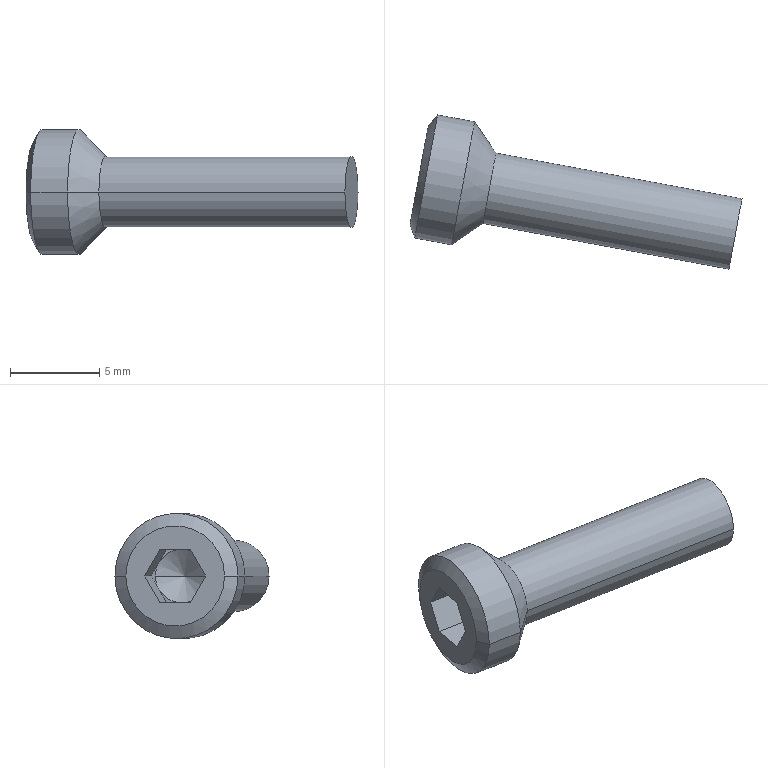Part | SolidWorks | features BaseBody 1 | 1 solid | 24 faces | box 18.575 x 8.622 x 7 mm | volume 288.186 mm3 | plane 14 | cone 6 | cylinder 4 | commonest cylinder face diameters 4 x2 7 x2
STEP:
#1=CARTESIAN_POINT('',(-115.606,1844.083,78.9));
#2=VERTEX_POINT('',#1);
#3=CARTESIAN_POINT('',(-114.875,1848.016,78.9));
#4=VERTEX_POINT('',#3);
#5=CARTESIAN_POINT('',(-115.241,1846.05,78.9));
#6=DIRECTION('',(-0.9832,0.1826,0.));
#7=DIRECTION('',(-0.1826,-0.9832,0.));
#8=AXIS2_PLACEMENT_3D('',#5,#6,#7);
#9=CIRCLE('',#8,2.);
#10=EDGE_CURVE('',#2,#4,#9,.T.);
#11=ORIENTED_EDGE('',*,*,#10,.T.);
#12=CARTESIAN_POINT('',(-128.64,1850.573,78.9));
#13=VERTEX_POINT('',#12);
#14=CARTESIAN_POINT('',(-132.573,1851.303,78.9));
#15=DIRECTION('',(-0.9832,0.1826,0.));
#16=VECTOR('',#15,1000.);
#17=LINE('',#14,#16);
#18=EDGE_CURVE('',#4,#13,#17,.T.);
#19=ORIENTED_EDGE('',*,*,#18,.T.);
#20=CARTESIAN_POINT('',(-129.37,1846.64,78.9));
#21=VERTEX_POINT('',#20);
#22=CARTESIAN_POINT('',(-129.005,1848.607,78.9));
#23=DIRECTION('',(0.9832,-0.1826,0.));
#24=DIRECTION('',(-0.1826,-0.9832,0.));
#25=AXIS2_PLACEMENT_3D('',#22,#23,#24);
#26=CIRCLE('',#25,2.);
#27=EDGE_CURVE('',#13,#21,#26,.T.);
#28=ORIENTED_EDGE('',*,*,#27,.T.);
#29=CARTESIAN_POINT('',(-133.303,1847.371,78.9));
#30=DIRECTION('',(-0.9832,0.1826,0.));
#31=VECTOR('',#30,1000.);
#32=LINE('',#29,#31);
#33=EDGE_CURVE('',#2,#21,#32,.T.);
#34=ORIENTED_EDGE('',*,*,#33,.F.);
#35=EDGE_LOOP('',(#11,#19,#28,#34));
#36=FACE_OUTER_BOUND('',#35,.T.);
#37=CARTESIAN_POINT('',(-132.938,1849.337,78.9));
#38=DIRECTION('',(-0.9832,0.1826,0.));
#39=DIRECTION('',(-0.1826,-0.9832,0.));
#40=AXIS2_PLACEMENT_3D('',#37,#38,#39);
#41=CYLINDRICAL_SURFACE('',#40,2.);
#42=ADVANCED_FACE('',(#36),#41,.T.);
#43=ORIENTED_EDGE('',*,*,#27,.F.);
#44=CARTESIAN_POINT('',(-129.841,1852.322,78.9));
#45=VERTEX_POINT('',#44);
#46=CARTESIAN_POINT('',(-129.841,1852.322,78.9));
#47=DIRECTION('',(-0.5661,0.8244,0.));
#48=VECTOR('',#47,1000.);
#49=LINE('',#46,#48);
#50=EDGE_CURVE('',#13,#45,#49,.T.);
#51=ORIENTED_EDGE('',*,*,#50,.T.);
#52=CARTESIAN_POINT('',(-131.119,1845.439,78.9));
#53=VERTEX_POINT('',#52);
#54=CARTESIAN_POINT('',(-130.48,1848.881,78.9));
#55=DIRECTION('',(0.9832,-0.1826,0.));
#56=DIRECTION('',(-0.1826,-0.9832,0.));
#57=AXIS2_PLACEMENT_3D('',#54,#55,#56);
#58=CIRCLE('',#57,3.5);
#59=EDGE_CURVE('',#45,#53,#58,.T.);
#60=ORIENTED_EDGE('',*,*,#59,.T.);
#61=CARTESIAN_POINT('',(-131.119,1845.439,78.9));
#62=DIRECTION('',(-0.8244,-0.5661,0.));
#63=VECTOR('',#62,1000.);
#64=LINE('',#61,#63);
#65=EDGE_CURVE('',#21,#53,#64,.T.);
#66=ORIENTED_EDGE('',*,*,#65,.F.);
#67=EDGE_LOOP('',(#43,#51,#60,#66));
#68=FACE_OUTER_BOUND('',#67,.T.);
#69=CARTESIAN_POINT('',(-130.48,1848.881,78.9));
#70=DIRECTION('',(-0.9832,0.1826,0.));
#71=DIRECTION('',(-0.1826,-0.9832,0.));
#72=AXIS2_PLACEMENT_3D('',#69,#70,#71);
#73=CONICAL_SURFACE('',#72,3.5,0.7854);
#74=ADVANCED_FACE('',(#68),#73,.T.);
#75=ORIENTED_EDGE('',*,*,#59,.F.);
#76=CARTESIAN_POINT('',(-131.905,1852.705,78.9));
#77=VERTEX_POINT('',#76);
#78=CARTESIAN_POINT('',(-132.299,1852.778,78.9));
#79=DIRECTION('',(-0.9832,0.1826,0.));
#80=VECTOR('',#79,1000.);
#81=LINE('',#78,#80);
#82=EDGE_CURVE('',#45,#77,#81,.T.);
#83=ORIENTED_EDGE('',*,*,#82,.T.);
#84=CARTESIAN_POINT('',(-133.184,1845.823,78.9));
#85=VERTEX_POINT('',#84);
#86=CARTESIAN_POINT('',(-132.545,1849.264,78.9));
#87=DIRECTION('',(0.9832,-0.1826,0.));
#88=DIRECTION('',(-0.1826,-0.9832,0.));
#89=AXIS2_PLACEMENT_3D('',#86,#87,#88);
#90=CIRCLE('',#89,3.5);
#91=EDGE_CURVE('',#77,#85,#90,.T.);
#92=ORIENTED_EDGE('',*,*,#91,.T.);
#93=CARTESIAN_POINT('',(-133.577,1845.896,78.9));
#94=DIRECTION('',(-0.9832,0.1826,0.));
#95=VECTOR('',#94,1000.);
#96=LINE('',#93,#95);
#97=EDGE_CURVE('',#53,#85,#96,.T.);
#98=ORIENTED_EDGE('',*,*,#97,.F.);
#99=EDGE_LOOP('',(#75,#83,#92,#98));
#100=FACE_OUTER_BOUND('',#99,.T.);
#101=CARTESIAN_POINT('',(-132.938,1849.337,78.9));
#102=DIRECTION('',(-0.9832,0.1826,0.));
#103=DIRECTION('',(-0.1826,-0.9832,0.));
#104=AXIS2_PLACEMENT_3D('',#101,#102,#103);
#105=CYLINDRICAL_SURFACE('',#104,3.5);
#106=ADVANCED_FACE('',(#100),#105,.T.);
#107=CARTESIAN_POINT('',(-132.425,1852.097,78.9));
#108=VERTEX_POINT('',#107);
#109=CARTESIAN_POINT('',(-133.451,1846.577,78.9));
#110=VERTEX_POINT('',#109);
#111=CARTESIAN_POINT('',(-132.938,1849.337,78.9));
#112=DIRECTION('',(0.9832,-0.1826,0.));
#113=DIRECTION('',(0.1826,0.9832,0.));
#114=AXIS2_PLACEMENT_3D('',#111,#112,#113);
#115=CIRCLE('',#114,2.807);
#116=EDGE_CURVE('',#108,#110,#115,.T.);
#117=ORIENTED_EDGE('',*,*,#116,.T.);
#118=CARTESIAN_POINT('',(-133.184,1845.823,78.9));
#119=DIRECTION('',(0.3334,-0.9428,0.));
#120=VECTOR('',#119,1000.);
#121=LINE('',#118,#120);
#122=EDGE_CURVE('',#110,#85,#121,.T.);
#123=ORIENTED_EDGE('',*,*,#122,.T.);
#124=ORIENTED_EDGE('',*,*,#91,.F.);
#125=CARTESIAN_POINT('',(-131.905,1852.705,78.9));
#126=DIRECTION('',(0.6497,0.7601,0.));
#127=VECTOR('',#126,1000.);
#128=LINE('',#125,#127);
#129=EDGE_CURVE('',#108,#77,#128,.T.);
#130=ORIENTED_EDGE('',*,*,#129,.F.);
#131=EDGE_LOOP('',(#117,#123,#124,#130));
#132=FACE_OUTER_BOUND('',#131,.T.);
#133=CARTESIAN_POINT('',(-132.545,1849.264,78.9));
#134=DIRECTION('',(0.9832,-0.1826,0.));
#135=DIRECTION('',(0.1826,0.9832,0.));
#136=AXIS2_PLACEMENT_3D('',#133,#134,#135);
#137=CONICAL_SURFACE('',#136,3.5,1.047);
#138=ADVANCED_FACE('',(#132),#137,.T.);
#139=CARTESIAN_POINT('',(-130.12,1848.814,78.9));
#140=VERTEX_POINT('',#139);
#141=CARTESIAN_POINT('',(-131.245,1847.497,78.9));
#142=VERTEX_POINT('',#141);
#143=CARTESIAN_POINT('',(-131.245,1847.497,78.9));
#144=DIRECTION('',(-0.6497,-0.7601,0.));
#145=VECTOR('',#144,1000.);
#146=LINE('',#143,#145);
#147=EDGE_CURVE('',#140,#142,#146,.T.);
#148=ORIENTED_EDGE('',*,*,#147,.F.);
#149=CARTESIAN_POINT('',(-130.698,1850.447,78.9));
#150=VERTEX_POINT('',#149);
#151=CARTESIAN_POINT('',(-130.698,1850.447,78.9));
#152=DIRECTION('',(-0.3334,0.9428,0.));
#153=VECTOR('',#152,1000.);
#154=LINE('',#151,#153);
#155=EDGE_CURVE('',#140,#150,#154,.T.);
#156=ORIENTED_EDGE('',*,*,#155,.T.);
#157=CARTESIAN_POINT('',(-130.734,1850.249,78.15));
#158=VERTEX_POINT('',#157);
#159=CARTESIAN_POINT('',(-130.971,1848.972,78.9));
#160=DIRECTION('',(0.9832,-0.1826,0.));
#161=DIRECTION('',(-0.1826,-0.9832,0.));
#162=AXIS2_PLACEMENT_3D('',#159,#160,#161);
#163=CIRCLE('',#162,1.5);
#164=EDGE_CURVE('',#158,#150,#163,.T.);
#165=ORIENTED_EDGE('',*,*,#164,.F.);
#166=CARTESIAN_POINT('',(-130.971,1848.972,77.4));
#167=VERTEX_POINT('',#166);
#168=CARTESIAN_POINT('',(-130.971,1848.972,78.9));
#169=DIRECTION('',(0.9832,-0.1826,0.));
#170=DIRECTION('',(-0.1826,-0.9832,0.));
#171=AXIS2_PLACEMENT_3D('',#168,#169,#170);
#172=CIRCLE('',#171,1.5);
#173=EDGE_CURVE('',#167,#158,#172,.T.);
#174=ORIENTED_EDGE('',*,*,#173,.F.);
#175=CARTESIAN_POINT('',(-131.209,1847.695,78.15));
#176=VERTEX_POINT('',#175);
#177=CARTESIAN_POINT('',(-130.971,1848.972,78.9));
#178=DIRECTION('',(0.9832,-0.1826,0.));
#179=DIRECTION('',(-0.1826,-0.9832,0.));
#180=AXIS2_PLACEMENT_3D('',#177,#178,#179);
#181=CIRCLE('',#180,1.5);
#182=EDGE_CURVE('',#176,#167,#181,.T.);
#183=ORIENTED_EDGE('',*,*,#182,.F.);
#184=CARTESIAN_POINT('',(-130.971,1848.972,78.9));
#185=DIRECTION('',(0.9832,-0.1826,0.));
#186=DIRECTION('',(-0.1826,-0.9832,0.));
#187=AXIS2_PLACEMENT_3D('',#184,#185,#186);
#188=CIRCLE('',#187,1.5);
#189=EDGE_CURVE('',#142,#176,#188,.T.);
#190=ORIENTED_EDGE('',*,*,#189,.F.);
#191=EDGE_LOOP('',(#148,#156,#165,#174,#183,#190));
#192=FACE_OUTER_BOUND('',#191,.T.);
#193=CARTESIAN_POINT('',(-130.971,1848.972,78.9));
#194=DIRECTION('',(-0.9832,0.1826,0.));
#195=DIRECTION('',(-0.1826,-0.9832,0.));
#196=AXIS2_PLACEMENT_3D('',#193,#194,#195);
#197=CONICAL_SURFACE('',#196,1.5,1.047);
#198=ADVANCED_FACE('',(#192),#197,.F.);
#199=ORIENTED_EDGE('',*,*,#18,.F.);
#200=CARTESIAN_POINT('',(-115.241,1846.05,78.9));
#201=DIRECTION('',(-0.9832,0.1826,0.));
#202=DIRECTION('',(-0.1826,-0.9832,0.));
#203=AXIS2_PLACEMENT_3D('',#200,#201,#202);
#204=CIRCLE('',#203,2.);
#205=EDGE_CURVE('',#4,#2,#204,.T.);
#206=ORIENTED_EDGE('',*,*,#205,.T.);
#207=ORIENTED_EDGE('',*,*,#33,.T.);
#208=CARTESIAN_POINT('',(-129.005,1848.607,78.9));
#209=DIRECTION('',(0.9832,-0.1826,0.));
#210=DIRECTION('',(-0.1826,-0.9832,0.));
#211=AXIS2_PLACEMENT_3D('',#208,#209,#210);
#212=CIRCLE('',#211,2.);
#213=EDGE_CURVE('',#21,#13,#212,.T.);
#214=ORIENTED_EDGE('',*,*,#213,.T.);
#215=EDGE_LOOP('',(#199,#206,#207,#214));
#216=FACE_OUTER_BOUND('',#215,.T.);
#217=CARTESIAN_POINT('',(-132.938,1849.337,78.9));
#218=DIRECTION('',(-0.9832,0.1826,0.));
#219=DIRECTION('',(-0.1826,-0.9832,0.));
#220=AXIS2_PLACEMENT_3D('',#217,#218,#219);
#221=CYLINDRICAL_SURFACE('',#220,2.);
#222=ADVANCED_FACE('',(#216),#221,.T.);
#223=ORIENTED_EDGE('',*,*,#50,.F.);
#224=ORIENTED_EDGE('',*,*,#213,.F.);
#225=ORIENTED_EDGE('',*,*,#65,.T.);
#226=CARTESIAN_POINT('',(-130.48,1848.881,78.9));
#227=DIRECTION('',(0.9832,-0.1826,0.));
#228=DIRECTION('',(-0.1826,-0.9832,0.));
#229=AXIS2_PLACEMENT_3D('',#226,#227,#228);
#230=CIRCLE('',#229,3.5);
#231=EDGE_CURVE('',#53,#45,#230,.T.);
#232=ORIENTED_EDGE('',*,*,#231,.T.);
#233=EDGE_LOOP('',(#223,#224,#225,#232));
#234=FACE_OUTER_BOUND('',#233,.T.);
#235=CARTESIAN_POINT('',(-130.48,1848.881,78.9));
#236=DIRECTION('',(-0.9832,0.1826,0.));
#237=DIRECTION('',(-0.1826,-0.9832,0.));
#238=AXIS2_PLACEMENT_3D('',#235,#236,#237);
#239=CONICAL_SURFACE('',#238,3.5,0.7854);
#240=ADVANCED_FACE('',(#234),#239,.T.);
#241=ORIENTED_EDGE('',*,*,#10,.F.);
#242=ORIENTED_EDGE('',*,*,#205,.F.);
#243=EDGE_LOOP('',(#241,#242));
#244=FACE_OUTER_BOUND('',#243,.T.);
#245=CARTESIAN_POINT('',(-114.875,1848.016,78.9));
#246=DIRECTION('',(-0.9832,0.1826,0.));
#247=DIRECTION('',(-0.1826,-0.9832,0.));
#248=AXIS2_PLACEMENT_3D('',#245,#246,#247);
#249=PLANE('',#248);
#250=ADVANCED_FACE('',(#244),#249,.F.);
#251=ORIENTED_EDGE('',*,*,#82,.F.);
#252=ORIENTED_EDGE('',*,*,#231,.F.);
#253=ORIENTED_EDGE('',*,*,#97,.T.);
#254=CARTESIAN_POINT('',(-132.545,1849.264,78.9));
#255=DIRECTION('',(0.9832,-0.1826,0.));
#256=DIRECTION('',(-0.1826,-0.9832,0.));
#257=AXIS2_PLACEMENT_3D('',#254,#255,#256);
#258=CIRCLE('',#257,3.5);
#259=EDGE_CURVE('',#85,#77,#258,.T.);
#260=ORIENTED_EDGE('',*,*,#259,.T.);
#261=EDGE_LOOP('',(#251,#252,#253,#260));
#262=FACE_OUTER_BOUND('',#261,.T.);
#263=CARTESIAN_POINT('',(-132.938,1849.337,78.9));
#264=DIRECTION('',(-0.9832,0.1826,0.));
#265=DIRECTION('',(-0.1826,-0.9832,0.));
#266=AXIS2_PLACEMENT_3D('',#263,#264,#265);
#267=CYLINDRICAL_SURFACE('',#266,3.5);
#268=ADVANCED_FACE('',(#262),#267,.T.);
#269=ORIENTED_EDGE('',*,*,#122,.F.);
#270=CARTESIAN_POINT('',(-132.938,1849.337,78.9));
#271=DIRECTION('',(0.9832,-0.1826,0.));
#272=DIRECTION('',(0.1826,0.9832,0.));
#273=AXIS2_PLACEMENT_3D('',#270,#271,#272);
#274=CIRCLE('',#273,2.807);
#275=EDGE_CURVE('',#110,#108,#274,.T.);
#276=ORIENTED_EDGE('',*,*,#275,.T.);
#277=ORIENTED_EDGE('',*,*,#129,.T.);
#278=ORIENTED_EDGE('',*,*,#259,.F.);
#279=EDGE_LOOP('',(#269,#276,#277,#278));
#280=FACE_OUTER_BOUND('',#279,.T.);
#281=CARTESIAN_POINT('',(-132.545,1849.264,78.9));
#282=DIRECTION('',(0.9832,-0.1826,0.));
#283=DIRECTION('',(0.1826,0.9832,0.));
#284=AXIS2_PLACEMENT_3D('',#281,#282,#283);
#285=CONICAL_SURFACE('',#284,3.5,1.047);
#286=ADVANCED_FACE('',(#280),#285,.T.);
#287=CARTESIAN_POINT('',(-133.096,1848.486,80.4));
#288=VERTEX_POINT('',#287);
#289=CARTESIAN_POINT('',(-132.78,1850.189,80.4));
#290=VERTEX_POINT('',#289);
#291=CARTESIAN_POINT('',(-132.938,1849.337,80.4));
#292=DIRECTION('',(0.1826,0.9832,0.));
#293=VECTOR('',#292,1000.);
#294=LINE('',#291,#293);
#295=EDGE_CURVE('',#288,#290,#294,.T.);
#296=ORIENTED_EDGE('',*,*,#295,.F.);
#297=CARTESIAN_POINT('',(-133.254,1847.634,78.9));
#298=VERTEX_POINT('',#297);
#299=CARTESIAN_POINT('',(-133.254,1847.634,78.9));
#300=DIRECTION('',(0.09131,0.4916,0.866));
#301=VECTOR('',#300,1000.);
#302=LINE('',#299,#301);
#303=EDGE_CURVE('',#298,#288,#302,.T.);
#304=ORIENTED_EDGE('',*,*,#303,.F.);
#305=CARTESIAN_POINT('',(-133.096,1848.486,77.4));
#306=VERTEX_POINT('',#305);
#307=CARTESIAN_POINT('',(-133.096,1848.486,77.4));
#308=DIRECTION('',(-0.09131,-0.4916,0.866));
#309=VECTOR('',#308,1000.);
#310=LINE('',#307,#309);
#311=EDGE_CURVE('',#306,#298,#310,.T.);
#312=ORIENTED_EDGE('',*,*,#311,.F.);
#313=CARTESIAN_POINT('',(-132.78,1850.189,77.4));
#314=VERTEX_POINT('',#313);
#315=CARTESIAN_POINT('',(-132.938,1849.337,77.4));
#316=DIRECTION('',(-0.1826,-0.9832,0.));
#317=VECTOR('',#316,1000.);
#318=LINE('',#315,#317);
#319=EDGE_CURVE('',#314,#306,#318,.T.);
#320=ORIENTED_EDGE('',*,*,#319,.F.);
#321=CARTESIAN_POINT('',(-132.622,1851.04,78.9));
#322=VERTEX_POINT('',#321);
#323=CARTESIAN_POINT('',(-132.622,1851.04,78.9));
#324=DIRECTION('',(-0.09131,-0.4916,-0.866));
#325=VECTOR('',#324,1000.);
#326=LINE('',#323,#325);
#327=EDGE_CURVE('',#322,#314,#326,.T.);
#328=ORIENTED_EDGE('',*,*,#327,.F.);
#329=CARTESIAN_POINT('',(-132.78,1850.189,80.4));
#330=DIRECTION('',(0.09131,0.4916,-0.866));
#331=VECTOR('',#330,1000.);
#332=LINE('',#329,#331);
#333=EDGE_CURVE('',#290,#322,#332,.T.);
#334=ORIENTED_EDGE('',*,*,#333,.F.);
#335=EDGE_LOOP('',(#296,#304,#312,#320,#328,#334));
#336=FACE_BOUND('',#335,.T.);
#337=ORIENTED_EDGE('',*,*,#116,.F.);
#338=ORIENTED_EDGE('',*,*,#275,.F.);
#339=EDGE_LOOP('',(#337,#338));
#340=FACE_OUTER_BOUND('',#339,.T.);
#341=CARTESIAN_POINT('',(-132.938,1849.337,78.9));
#342=DIRECTION('',(0.9832,-0.1826,0.));
#343=DIRECTION('',(0.1826,0.9832,0.));
#344=AXIS2_PLACEMENT_3D('',#341,#342,#343);
#345=PLANE('',#344);
#346=ADVANCED_FACE('',(#336,#340),#345,.F.);
#347=CARTESIAN_POINT('',(-130.734,1850.249,79.65));
#348=VERTEX_POINT('',#347);
#349=CARTESIAN_POINT('',(-130.655,1850.675,78.9));
#350=VERTEX_POINT('',#349);
#351=CARTESIAN_POINT('',(-130.734,1850.249,79.65));
#352=DIRECTION('',(0.09131,0.4916,-0.866));
#353=VECTOR('',#352,1000.);
#354=LINE('',#351,#353);
#355=EDGE_CURVE('',#348,#350,#354,.T.);
#356=ORIENTED_EDGE('',*,*,#355,.F.);
#357=CARTESIAN_POINT('',(-130.813,1849.823,80.4));
#358=VERTEX_POINT('',#357);
#359=CARTESIAN_POINT('',(-130.813,1849.823,80.4));
#360=DIRECTION('',(0.09131,0.4916,-0.866));
#361=VECTOR('',#360,1000.);
#362=LINE('',#359,#361);
#363=EDGE_CURVE('',#358,#348,#362,.T.);
#364=ORIENTED_EDGE('',*,*,#363,.F.);
#365=CARTESIAN_POINT('',(-132.78,1850.189,80.4));
#366=DIRECTION('',(0.9832,-0.1826,0.));
#367=VECTOR('',#366,1000.);
#368=LINE('',#365,#367);
#369=EDGE_CURVE('',#290,#358,#368,.T.);
#370=ORIENTED_EDGE('',*,*,#369,.F.);
#371=ORIENTED_EDGE('',*,*,#333,.T.);
#372=CARTESIAN_POINT('',(-130.655,1850.675,78.9));
#373=DIRECTION('',(-0.9832,0.1826,0.));
#374=VECTOR('',#373,1000.);
#375=LINE('',#372,#374);
#376=EDGE_CURVE('',#350,#322,#375,.T.);
#377=ORIENTED_EDGE('',*,*,#376,.F.);
#378=EDGE_LOOP('',(#356,#364,#370,#371,#377));
#379=FACE_OUTER_BOUND('',#378,.T.);
#380=CARTESIAN_POINT('',(-130.813,1849.823,80.4));
#381=DIRECTION('',(0.1582,0.8515,0.5));
#382=DIRECTION('',(0.,-0.5064,0.8623));
#383=AXIS2_PLACEMENT_3D('',#380,#381,#382);
#384=PLANE('',#383);
#385=ADVANCED_FACE('',(#379),#384,.F.);
#386=CARTESIAN_POINT('',(-130.971,1848.972,80.4));
#387=VERTEX_POINT('',#386);
#388=CARTESIAN_POINT('',(-130.971,1848.972,80.4));
#389=DIRECTION('',(0.1826,0.9832,0.));
#390=VECTOR('',#389,1000.);
#391=LINE('',#388,#390);
#392=EDGE_CURVE('',#387,#358,#391,.T.);
#393=ORIENTED_EDGE('',*,*,#392,.F.);
#394=CARTESIAN_POINT('',(-131.13,1848.12,80.4));
#395=VERTEX_POINT('',#394);
#396=CARTESIAN_POINT('',(-131.13,1848.12,80.4));
#397=DIRECTION('',(0.1826,0.9832,0.));
#398=VECTOR('',#397,1000.);
#399=LINE('',#396,#398);
#400=EDGE_CURVE('',#395,#387,#399,.T.);
#401=ORIENTED_EDGE('',*,*,#400,.F.);
#402=CARTESIAN_POINT('',(-133.096,1848.486,80.4));
#403=DIRECTION('',(0.9832,-0.1826,0.));
#404=VECTOR('',#403,1000.);
#405=LINE('',#402,#404);
#406=EDGE_CURVE('',#288,#395,#405,.T.);
#407=ORIENTED_EDGE('',*,*,#406,.F.);
#408=ORIENTED_EDGE('',*,*,#295,.T.);
#409=ORIENTED_EDGE('',*,*,#369,.T.);
#410=EDGE_LOOP('',(#393,#401,#407,#408,#409));
#411=FACE_OUTER_BOUND('',#410,.T.);
#412=CARTESIAN_POINT('',(-131.13,1848.12,80.4));
#413=DIRECTION('',(0.,0.,1.));
#414=DIRECTION('',(1.,0.,0.));
#415=AXIS2_PLACEMENT_3D('',#412,#413,#414);
#416=PLANE('',#415);
#417=ADVANCED_FACE('',(#411),#416,.F.);
#418=CARTESIAN_POINT('',(-131.209,1847.695,79.65));
#419=VERTEX_POINT('',#418);
#420=CARTESIAN_POINT('',(-131.209,1847.695,79.65));
#421=DIRECTION('',(0.09131,0.4916,0.866));
#422=VECTOR('',#421,1000.);
#423=LINE('',#420,#422);
#424=EDGE_CURVE('',#419,#395,#423,.T.);
#425=ORIENTED_EDGE('',*,*,#424,.F.);
#426=CARTESIAN_POINT('',(-131.288,1847.269,78.9));
#427=VERTEX_POINT('',#426);
#428=CARTESIAN_POINT('',(-131.288,1847.269,78.9));
#429=DIRECTION('',(0.09131,0.4916,0.866));
#430=VECTOR('',#429,1000.);
#431=LINE('',#428,#430);
#432=EDGE_CURVE('',#427,#419,#431,.T.);
#433=ORIENTED_EDGE('',*,*,#432,.F.);
#434=CARTESIAN_POINT('',(-133.254,1847.634,78.9));
#435=DIRECTION('',(0.9832,-0.1826,0.));
#436=VECTOR('',#435,1000.);
#437=LINE('',#434,#436);
#438=EDGE_CURVE('',#298,#427,#437,.T.);
#439=ORIENTED_EDGE('',*,*,#438,.F.);
#440=ORIENTED_EDGE('',*,*,#303,.T.);
#441=ORIENTED_EDGE('',*,*,#406,.T.);
#442=EDGE_LOOP('',(#425,#433,#439,#440,#441));
#443=FACE_OUTER_BOUND('',#442,.T.);
#444=CARTESIAN_POINT('',(-131.288,1847.269,78.9));
#445=DIRECTION('',(-0.1582,-0.8515,0.5));
#446=DIRECTION('',(0.,-0.5064,-0.8623));
#447=AXIS2_PLACEMENT_3D('',#444,#445,#446);
#448=PLANE('',#447);
#449=ADVANCED_FACE('',(#443),#448,.F.);
#450=CARTESIAN_POINT('',(-131.209,1847.695,78.15));
#451=DIRECTION('',(-0.09131,-0.4916,0.866));
#452=VECTOR('',#451,1000.);
#453=LINE('',#450,#452);
#454=EDGE_CURVE('',#176,#427,#453,.T.);
#455=ORIENTED_EDGE('',*,*,#454,.F.);
#456=CARTESIAN_POINT('',(-131.13,1848.12,77.4));
#457=VERTEX_POINT('',#456);
#458=CARTESIAN_POINT('',(-131.13,1848.12,77.4));
#459=DIRECTION('',(-0.09131,-0.4916,0.866));
#460=VECTOR('',#459,1000.);
#461=LINE('',#458,#460);
#462=EDGE_CURVE('',#457,#176,#461,.T.);
#463=ORIENTED_EDGE('',*,*,#462,.F.);
#464=CARTESIAN_POINT('',(-133.096,1848.486,77.4));
#465=DIRECTION('',(0.9832,-0.1826,0.));
#466=VECTOR('',#465,1000.);
#467=LINE('',#464,#466);
#468=EDGE_CURVE('',#306,#457,#467,.T.);
#469=ORIENTED_EDGE('',*,*,#468,.F.);
#470=ORIENTED_EDGE('',*,*,#311,.T.);
#471=ORIENTED_EDGE('',*,*,#438,.T.);
#472=EDGE_LOOP('',(#455,#463,#469,#470,#471));
#473=FACE_OUTER_BOUND('',#472,.T.);
#474=CARTESIAN_POINT('',(-131.13,1848.12,77.4));
#475=DIRECTION('',(-0.1582,-0.8515,-0.5));
#476=DIRECTION('',(0.,0.5064,-0.8623));
#477=AXIS2_PLACEMENT_3D('',#474,#475,#476);
#478=PLANE('',#477);
#479=ADVANCED_FACE('',(#473),#478,.F.);
#480=CARTESIAN_POINT('',(-130.971,1848.972,77.4));
#481=DIRECTION('',(-0.1826,-0.9832,0.));
#482=VECTOR('',#481,1000.);
#483=LINE('',#480,#482);
#484=EDGE_CURVE('',#167,#457,#483,.T.);
#485=ORIENTED_EDGE('',*,*,#484,.F.);
#486=CARTESIAN_POINT('',(-130.813,1849.823,77.4));
#487=VERTEX_POINT('',#486);
#488=CARTESIAN_POINT('',(-130.813,1849.823,77.4));
#489=DIRECTION('',(-0.1826,-0.9832,0.));
#490=VECTOR('',#489,1000.);
#491=LINE('',#488,#490);
#492=EDGE_CURVE('',#487,#167,#491,.T.);
#493=ORIENTED_EDGE('',*,*,#492,.F.);
#494=CARTESIAN_POINT('',(-132.78,1850.189,77.4));
#495=DIRECTION('',(0.9832,-0.1826,0.));
#496=VECTOR('',#495,1000.);
#497=LINE('',#494,#496);
#498=EDGE_CURVE('',#314,#487,#497,.T.);
#499=ORIENTED_EDGE('',*,*,#498,.F.);
#500=ORIENTED_EDGE('',*,*,#319,.T.);
#501=ORIENTED_EDGE('',*,*,#468,.T.);
#502=EDGE_LOOP('',(#485,#493,#499,#500,#501));
#503=FACE_OUTER_BOUND('',#502,.T.);
#504=CARTESIAN_POINT('',(-130.813,1849.823,77.4));
#505=DIRECTION('',(0.,0.,-1.));
#506=DIRECTION('',(-1.,0.,0.));
#507=AXIS2_PLACEMENT_3D('',#504,#505,#506);
#508=PLANE('',#507);
#509=ADVANCED_FACE('',(#503),#508,.F.);
#510=CARTESIAN_POINT('',(-130.734,1850.249,78.15));
#511=DIRECTION('',(-0.09131,-0.4916,-0.866));
#512=VECTOR('',#511,1000.);
#513=LINE('',#510,#512);
#514=EDGE_CURVE('',#158,#487,#513,.T.);
#515=ORIENTED_EDGE('',*,*,#514,.F.);
#516=CARTESIAN_POINT('',(-130.655,1850.675,78.9));
#517=DIRECTION('',(-0.09131,-0.4916,-0.866));
#518=VECTOR('',#517,1000.);
#519=LINE('',#516,#518);
#520=EDGE_CURVE('',#350,#158,#519,.T.);
#521=ORIENTED_EDGE('',*,*,#520,.F.);
#522=ORIENTED_EDGE('',*,*,#376,.T.);
#523=ORIENTED_EDGE('',*,*,#327,.T.);
#524=ORIENTED_EDGE('',*,*,#498,.T.);
#525=EDGE_LOOP('',(#515,#521,#522,#523,#524));
#526=FACE_OUTER_BOUND('',#525,.T.);
#527=CARTESIAN_POINT('',(-130.655,1850.675,78.9));
#528=DIRECTION('',(0.1582,0.8515,-0.5));
#529=DIRECTION('',(0.,0.5064,0.8623));
#530=AXIS2_PLACEMENT_3D('',#527,#528,#529);
#531=PLANE('',#530);
#532=ADVANCED_FACE('',(#526),#531,.F.);
#533=ORIENTED_EDGE('',*,*,#520,.T.);
#534=ORIENTED_EDGE('',*,*,#164,.T.);
#535=CARTESIAN_POINT('',(-130.971,1848.972,78.9));
#536=DIRECTION('',(0.9832,-0.1826,0.));
#537=DIRECTION('',(-0.1826,-0.9832,0.));
#538=AXIS2_PLACEMENT_3D('',#535,#536,#537);
#539=CIRCLE('',#538,1.5);
#540=EDGE_CURVE('',#150,#348,#539,.T.);
#541=ORIENTED_EDGE('',*,*,#540,.T.);
#542=ORIENTED_EDGE('',*,*,#355,.T.);
#543=EDGE_LOOP('',(#533,#534,#541,#542));
#544=FACE_OUTER_BOUND('',#543,.T.);
#545=CARTESIAN_POINT('',(-130.971,1848.972,78.9));
#546=DIRECTION('',(-0.9832,0.1826,0.));
#547=DIRECTION('',(-0.1826,-0.9832,0.));
#548=AXIS2_PLACEMENT_3D('',#545,#546,#547);
#549=PLANE('',#548);
#550=ADVANCED_FACE('',(#544),#549,.T.);
#551=ORIENTED_EDGE('',*,*,#392,.T.);
#552=ORIENTED_EDGE('',*,*,#363,.T.);
#553=CARTESIAN_POINT('',(-130.971,1848.972,78.9));
#554=DIRECTION('',(0.9832,-0.1826,0.));
#555=DIRECTION('',(-0.1826,-0.9832,0.));
#556=AXIS2_PLACEMENT_3D('',#553,#554,#555);
#557=CIRCLE('',#556,1.5);
#558=EDGE_CURVE('',#348,#387,#557,.T.);
#559=ORIENTED_EDGE('',*,*,#558,.T.);
#560=EDGE_LOOP('',(#551,#552,#559));
#561=FACE_OUTER_BOUND('',#560,.T.);
#562=CARTESIAN_POINT('',(-130.971,1848.972,78.9));
#563=DIRECTION('',(-0.9832,0.1826,0.));
#564=DIRECTION('',(-0.1826,-0.9832,0.));
#565=AXIS2_PLACEMENT_3D('',#562,#563,#564);
#566=PLANE('',#565);
#567=ADVANCED_FACE('',(#561),#566,.T.);
#568=ORIENTED_EDGE('',*,*,#424,.T.);
#569=ORIENTED_EDGE('',*,*,#400,.T.);
#570=CARTESIAN_POINT('',(-130.971,1848.972,78.9));
#571=DIRECTION('',(0.9832,-0.1826,0.));
#572=DIRECTION('',(-0.1826,-0.9832,0.));
#573=AXIS2_PLACEMENT_3D('',#570,#571,#572);
#574=CIRCLE('',#573,1.5);
#575=EDGE_CURVE('',#387,#419,#574,.T.);
#576=ORIENTED_EDGE('',*,*,#575,.T.);
#577=EDGE_LOOP('',(#568,#569,#576));
#578=FACE_OUTER_BOUND('',#577,.T.);
#579=CARTESIAN_POINT('',(-130.971,1848.972,78.9));
#580=DIRECTION('',(-0.9832,0.1826,0.));
#581=DIRECTION('',(-0.1826,-0.9832,0.));
#582=AXIS2_PLACEMENT_3D('',#579,#580,#581);
#583=PLANE('',#582);
#584=ADVANCED_FACE('',(#578),#583,.T.);
#585=ORIENTED_EDGE('',*,*,#454,.T.);
#586=ORIENTED_EDGE('',*,*,#432,.T.);
#587=CARTESIAN_POINT('',(-130.971,1848.972,78.9));
#588=DIRECTION('',(0.9832,-0.1826,0.));
#589=DIRECTION('',(-0.1826,-0.9832,0.));
#590=AXIS2_PLACEMENT_3D('',#587,#588,#589);
#591=CIRCLE('',#590,1.5);
#592=EDGE_CURVE('',#419,#142,#591,.T.);
#593=ORIENTED_EDGE('',*,*,#592,.T.);
#594=ORIENTED_EDGE('',*,*,#189,.T.);
#595=EDGE_LOOP('',(#585,#586,#593,#594));
#596=FACE_OUTER_BOUND('',#595,.T.);
#597=CARTESIAN_POINT('',(-130.971,1848.972,78.9));
#598=DIRECTION('',(-0.9832,0.1826,0.));
#599=DIRECTION('',(-0.1826,-0.9832,0.));
#600=AXIS2_PLACEMENT_3D('',#597,#598,#599);
#601=PLANE('',#600);
#602=ADVANCED_FACE('',(#596),#601,.T.);
#603=ORIENTED_EDGE('',*,*,#484,.T.);
#604=ORIENTED_EDGE('',*,*,#462,.T.);
#605=ORIENTED_EDGE('',*,*,#182,.T.);
#606=EDGE_LOOP('',(#603,#604,#605));
#607=FACE_OUTER_BOUND('',#606,.T.);
#608=CARTESIAN_POINT('',(-130.971,1848.972,78.9));
#609=DIRECTION('',(-0.9832,0.1826,0.));
#610=DIRECTION('',(-0.1826,-0.9832,0.));
#611=AXIS2_PLACEMENT_3D('',#608,#609,#610);
#612=PLANE('',#611);
#613=ADVANCED_FACE('',(#607),#612,.T.);
#614=ORIENTED_EDGE('',*,*,#514,.T.);
#615=ORIENTED_EDGE('',*,*,#492,.T.);
#616=ORIENTED_EDGE('',*,*,#173,.T.);
#617=EDGE_LOOP('',(#614,#615,#616));
#618=FACE_OUTER_BOUND('',#617,.T.);
#619=CARTESIAN_POINT('',(-130.971,1848.972,78.9));
#620=DIRECTION('',(-0.9832,0.1826,0.));
#621=DIRECTION('',(-0.1826,-0.9832,0.));
#622=AXIS2_PLACEMENT_3D('',#619,#620,#621);
#623=PLANE('',#622);
#624=ADVANCED_FACE('',(#618),#623,.T.);
#625=ORIENTED_EDGE('',*,*,#155,.F.);
#626=ORIENTED_EDGE('',*,*,#147,.T.);
#627=ORIENTED_EDGE('',*,*,#592,.F.);
#628=ORIENTED_EDGE('',*,*,#575,.F.);
#629=ORIENTED_EDGE('',*,*,#558,.F.);
#630=ORIENTED_EDGE('',*,*,#540,.F.);
#631=EDGE_LOOP('',(#625,#626,#627,#628,#629,#630));
#632=FACE_OUTER_BOUND('',#631,.T.);
#633=CARTESIAN_POINT('',(-130.971,1848.972,78.9));
#634=DIRECTION('',(-0.9832,0.1826,0.));
#635=DIRECTION('',(-0.1826,-0.9832,0.));
#636=AXIS2_PLACEMENT_3D('',#633,#634,#635);
#637=CONICAL_SURFACE('',#636,1.5,1.047);
#638=ADVANCED_FACE('',(#632),#637,.F.);
#639=CLOSED_SHELL('',(#42,#74,#106,#138,#198,#222,#240,#250,#268,#286,#346,#385,#417,#449,#479,#509,#532,#550,#567,#584,#602,#613,#624,#638));
#640=MANIFOLD_SOLID_BREP('',#639);
#641=CARTESIAN_POINT('',(0.,0.,0.));
#642=DIRECTION('',(0.,0.,1.));
#643=DIRECTION('',(1.,0.,0.));
#644=AXIS2_PLACEMENT_3D('',#641,#642,#643);
#645=(LENGTH_UNIT()NAMED_UNIT(*)SI_UNIT(.MILLI.,.METRE.));
#646=UNCERTAINTY_MEASURE_WITH_UNIT(LENGTH_MEASURE(0.00001),#645,'','');
#647=(NAMED_UNIT(*)PLANE_ANGLE_UNIT()SI_UNIT($,.RADIAN.));
#648=(NAMED_UNIT(*)SI_UNIT($,.STERADIAN.)SOLID_ANGLE_UNIT());
#649=(GEOMETRIC_REPRESENTATION_CONTEXT(3)GLOBAL_UNCERTAINTY_ASSIGNED_CONTEXT((#646))GLOBAL_UNIT_ASSIGNED_CONTEXT((#645,#647,#648))REPRESENTATION_CONTEXT('',''));
#650=ADVANCED_BREP_SHAPE_REPRESENTATION('',(#640,#644),#649);